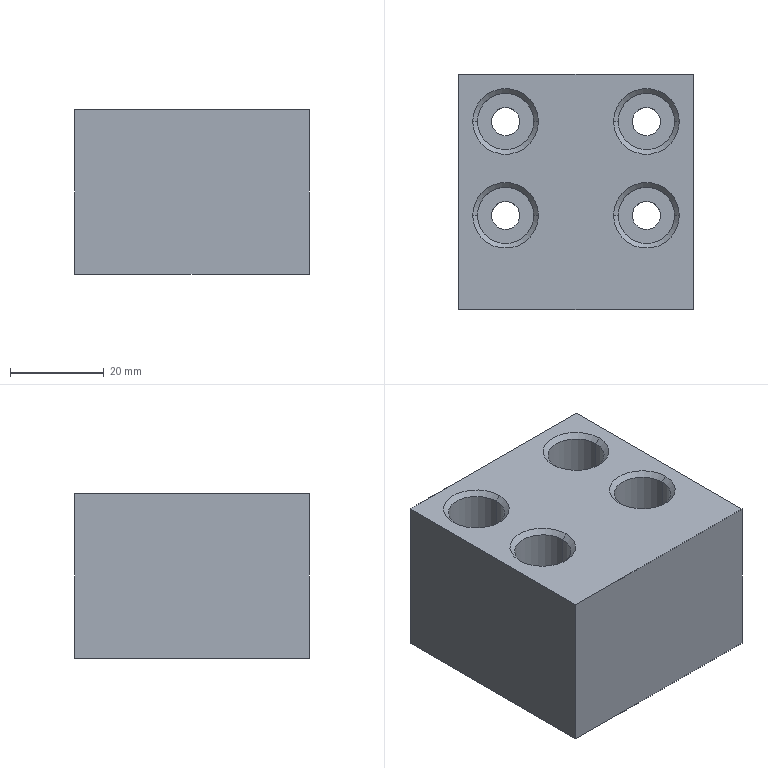Part | STEP file | Stopper | 1 solid | 42 faces | box 50 x 50 x 35 mm | volume 78331 mm3 | cone 16 | cylinder 16 | plane 10 | commonest cylinder face diameters 6 x8 12 x8
STEP:
#1=CARTESIAN_POINT('',(6.228,-22.942,1.));
#2=VERTEX_POINT('',#1);
#3=CARTESIAN_POINT('',(0.2277,-22.942,1.));
#4=VERTEX_POINT('',#3);
#5=CARTESIAN_POINT('',(3.228,-22.942,1.));
#6=DIRECTION('',(0.,0.,-1.));
#7=DIRECTION('',(-1.,0.,0.));
#8=AXIS2_PLACEMENT_3D('',#5,#6,#7);
#9=CIRCLE('',#8,3.);
#10=EDGE_CURVE('',#2,#4,#9,.T.);
#11=ORIENTED_EDGE('',*,*,#10,.F.);
#12=CARTESIAN_POINT('',(7.228,-22.942,0.));
#13=VERTEX_POINT('',#12);
#14=CARTESIAN_POINT('',(7.228,-22.942,0.));
#15=DIRECTION('',(0.7071,0.,-0.7071));
#16=VECTOR('',#15,1000.);
#17=LINE('',#14,#16);
#18=EDGE_CURVE('',#2,#13,#17,.T.);
#19=ORIENTED_EDGE('',*,*,#18,.T.);
#20=CARTESIAN_POINT('',(-0.7723,-22.942,0.));
#21=VERTEX_POINT('',#20);
#22=CARTESIAN_POINT('',(3.228,-22.942,0.));
#23=DIRECTION('',(0.,0.,-1.));
#24=DIRECTION('',(-1.,0.,0.));
#25=AXIS2_PLACEMENT_3D('',#22,#23,#24);
#26=CIRCLE('',#25,4.);
#27=EDGE_CURVE('',#13,#21,#26,.T.);
#28=ORIENTED_EDGE('',*,*,#27,.T.);
#29=CARTESIAN_POINT('',(-0.7723,-22.942,0.));
#30=DIRECTION('',(-0.7071,0.,-0.7071));
#31=VECTOR('',#30,1000.);
#32=LINE('',#29,#31);
#33=EDGE_CURVE('',#4,#21,#32,.T.);
#34=ORIENTED_EDGE('',*,*,#33,.F.);
#35=EDGE_LOOP('',(#11,#19,#28,#34));
#36=FACE_OUTER_BOUND('',#35,.T.);
#37=CARTESIAN_POINT('',(3.228,-22.942,0.));
#38=DIRECTION('',(0.,0.,-1.));
#39=DIRECTION('',(-1.,0.,0.));
#40=AXIS2_PLACEMENT_3D('',#37,#38,#39);
#41=CONICAL_SURFACE('',#40,4.,0.7854);
#42=ADVANCED_FACE('',(#36),#41,.F.);
#43=CARTESIAN_POINT('',(-23.772,-22.942,1.));
#44=VERTEX_POINT('',#43);
#45=CARTESIAN_POINT('',(-29.772,-22.942,1.));
#46=VERTEX_POINT('',#45);
#47=CARTESIAN_POINT('',(-26.772,-22.942,1.));
#48=DIRECTION('',(0.,0.,-1.));
#49=DIRECTION('',(-1.,0.,0.));
#50=AXIS2_PLACEMENT_3D('',#47,#48,#49);
#51=CIRCLE('',#50,3.);
#52=EDGE_CURVE('',#44,#46,#51,.T.);
#53=ORIENTED_EDGE('',*,*,#52,.F.);
#54=CARTESIAN_POINT('',(-22.772,-22.942,0.));
#55=VERTEX_POINT('',#54);
#56=CARTESIAN_POINT('',(-22.772,-22.942,0.));
#57=DIRECTION('',(0.7071,0.,-0.7071));
#58=VECTOR('',#57,1000.);
#59=LINE('',#56,#58);
#60=EDGE_CURVE('',#44,#55,#59,.T.);
#61=ORIENTED_EDGE('',*,*,#60,.T.);
#62=CARTESIAN_POINT('',(-30.772,-22.942,0.));
#63=VERTEX_POINT('',#62);
#64=CARTESIAN_POINT('',(-26.772,-22.942,0.));
#65=DIRECTION('',(0.,0.,-1.));
#66=DIRECTION('',(-1.,0.,0.));
#67=AXIS2_PLACEMENT_3D('',#64,#65,#66);
#68=CIRCLE('',#67,4.);
#69=EDGE_CURVE('',#55,#63,#68,.T.);
#70=ORIENTED_EDGE('',*,*,#69,.T.);
#71=CARTESIAN_POINT('',(-30.772,-22.942,0.));
#72=DIRECTION('',(-0.7071,0.,-0.7071));
#73=VECTOR('',#72,1000.);
#74=LINE('',#71,#73);
#75=EDGE_CURVE('',#46,#63,#74,.T.);
#76=ORIENTED_EDGE('',*,*,#75,.F.);
#77=EDGE_LOOP('',(#53,#61,#70,#76));
#78=FACE_OUTER_BOUND('',#77,.T.);
#79=CARTESIAN_POINT('',(-26.772,-22.942,0.));
#80=DIRECTION('',(0.,0.,-1.));
#81=DIRECTION('',(-1.,0.,0.));
#82=AXIS2_PLACEMENT_3D('',#79,#80,#81);
#83=CONICAL_SURFACE('',#82,4.,0.7854);
#84=ADVANCED_FACE('',(#78),#83,.F.);
#85=CARTESIAN_POINT('',(-23.772,-42.942,1.));
#86=VERTEX_POINT('',#85);
#87=CARTESIAN_POINT('',(-29.772,-42.942,1.));
#88=VERTEX_POINT('',#87);
#89=CARTESIAN_POINT('',(-26.772,-42.942,1.));
#90=DIRECTION('',(0.,0.,-1.));
#91=DIRECTION('',(-1.,0.,0.));
#92=AXIS2_PLACEMENT_3D('',#89,#90,#91);
#93=CIRCLE('',#92,3.);
#94=EDGE_CURVE('',#86,#88,#93,.T.);
#95=ORIENTED_EDGE('',*,*,#94,.F.);
#96=CARTESIAN_POINT('',(-22.772,-42.942,0.));
#97=VERTEX_POINT('',#96);
#98=CARTESIAN_POINT('',(-22.772,-42.942,0.));
#99=DIRECTION('',(0.7071,0.,-0.7071));
#100=VECTOR('',#99,1000.);
#101=LINE('',#98,#100);
#102=EDGE_CURVE('',#86,#97,#101,.T.);
#103=ORIENTED_EDGE('',*,*,#102,.T.);
#104=CARTESIAN_POINT('',(-30.772,-42.942,0.));
#105=VERTEX_POINT('',#104);
#106=CARTESIAN_POINT('',(-26.772,-42.942,0.));
#107=DIRECTION('',(0.,0.,-1.));
#108=DIRECTION('',(-1.,0.,0.));
#109=AXIS2_PLACEMENT_3D('',#106,#107,#108);
#110=CIRCLE('',#109,4.);
#111=EDGE_CURVE('',#97,#105,#110,.T.);
#112=ORIENTED_EDGE('',*,*,#111,.T.);
#113=CARTESIAN_POINT('',(-30.772,-42.942,0.));
#114=DIRECTION('',(-0.7071,0.,-0.7071));
#115=VECTOR('',#114,1000.);
#116=LINE('',#113,#115);
#117=EDGE_CURVE('',#88,#105,#116,.T.);
#118=ORIENTED_EDGE('',*,*,#117,.F.);
#119=EDGE_LOOP('',(#95,#103,#112,#118));
#120=FACE_OUTER_BOUND('',#119,.T.);
#121=CARTESIAN_POINT('',(-26.772,-42.942,0.));
#122=DIRECTION('',(0.,0.,-1.));
#123=DIRECTION('',(-1.,0.,0.));
#124=AXIS2_PLACEMENT_3D('',#121,#122,#123);
#125=CONICAL_SURFACE('',#124,4.,0.7854);
#126=ADVANCED_FACE('',(#120),#125,.F.);
#127=CARTESIAN_POINT('',(6.228,-42.942,1.));
#128=VERTEX_POINT('',#127);
#129=CARTESIAN_POINT('',(0.2277,-42.942,1.));
#130=VERTEX_POINT('',#129);
#131=CARTESIAN_POINT('',(3.228,-42.942,1.));
#132=DIRECTION('',(0.,0.,-1.));
#133=DIRECTION('',(-1.,0.,0.));
#134=AXIS2_PLACEMENT_3D('',#131,#132,#133);
#135=CIRCLE('',#134,3.);
#136=EDGE_CURVE('',#128,#130,#135,.T.);
#137=ORIENTED_EDGE('',*,*,#136,.F.);
#138=CARTESIAN_POINT('',(7.228,-42.942,0.));
#139=VERTEX_POINT('',#138);
#140=CARTESIAN_POINT('',(7.228,-42.942,0.));
#141=DIRECTION('',(0.7071,0.,-0.7071));
#142=VECTOR('',#141,1000.);
#143=LINE('',#140,#142);
#144=EDGE_CURVE('',#128,#139,#143,.T.);
#145=ORIENTED_EDGE('',*,*,#144,.T.);
#146=CARTESIAN_POINT('',(-0.7723,-42.942,0.));
#147=VERTEX_POINT('',#146);
#148=CARTESIAN_POINT('',(3.228,-42.942,0.));
#149=DIRECTION('',(0.,0.,-1.));
#150=DIRECTION('',(-1.,0.,0.));
#151=AXIS2_PLACEMENT_3D('',#148,#149,#150);
#152=CIRCLE('',#151,4.);
#153=EDGE_CURVE('',#139,#147,#152,.T.);
#154=ORIENTED_EDGE('',*,*,#153,.T.);
#155=CARTESIAN_POINT('',(-0.7723,-42.942,0.));
#156=DIRECTION('',(-0.7071,0.,-0.7071));
#157=VECTOR('',#156,1000.);
#158=LINE('',#155,#157);
#159=EDGE_CURVE('',#130,#147,#158,.T.);
#160=ORIENTED_EDGE('',*,*,#159,.F.);
#161=EDGE_LOOP('',(#137,#145,#154,#160));
#162=FACE_OUTER_BOUND('',#161,.T.);
#163=CARTESIAN_POINT('',(3.228,-42.942,0.));
#164=DIRECTION('',(0.,0.,-1.));
#165=DIRECTION('',(-1.,0.,0.));
#166=AXIS2_PLACEMENT_3D('',#163,#164,#165);
#167=CONICAL_SURFACE('',#166,4.,0.7854);
#168=ADVANCED_FACE('',(#162),#167,.F.);
#169=CARTESIAN_POINT('',(6.228,-22.942,20.));
#170=VERTEX_POINT('',#169);
#171=CARTESIAN_POINT('',(0.2277,-22.942,20.));
#172=VERTEX_POINT('',#171);
#173=CARTESIAN_POINT('',(3.228,-22.942,20.));
#174=DIRECTION('',(0.,0.,-1.));
#175=DIRECTION('',(-1.,0.,0.));
#176=AXIS2_PLACEMENT_3D('',#173,#174,#175);
#177=CIRCLE('',#176,3.);
#178=EDGE_CURVE('',#170,#172,#177,.T.);
#179=ORIENTED_EDGE('',*,*,#178,.F.);
#180=CARTESIAN_POINT('',(6.228,-22.942,35.));
#181=DIRECTION('',(0.,0.,-1.));
#182=VECTOR('',#181,1000.);
#183=LINE('',#180,#182);
#184=EDGE_CURVE('',#170,#2,#183,.T.);
#185=ORIENTED_EDGE('',*,*,#184,.T.);
#186=ORIENTED_EDGE('',*,*,#10,.T.);
#187=CARTESIAN_POINT('',(0.2277,-22.942,35.));
#188=DIRECTION('',(0.,0.,-1.));
#189=VECTOR('',#188,1000.);
#190=LINE('',#187,#189);
#191=EDGE_CURVE('',#172,#4,#190,.T.);
#192=ORIENTED_EDGE('',*,*,#191,.F.);
#193=EDGE_LOOP('',(#179,#185,#186,#192));
#194=FACE_OUTER_BOUND('',#193,.T.);
#195=CARTESIAN_POINT('',(3.228,-22.942,35.));
#196=DIRECTION('',(0.,0.,-1.));
#197=DIRECTION('',(-1.,0.,0.));
#198=AXIS2_PLACEMENT_3D('',#195,#196,#197);
#199=CYLINDRICAL_SURFACE('',#198,3.);
#200=ADVANCED_FACE('',(#194),#199,.F.);
#201=CARTESIAN_POINT('',(-23.772,-22.942,20.));
#202=VERTEX_POINT('',#201);
#203=CARTESIAN_POINT('',(-29.772,-22.942,20.));
#204=VERTEX_POINT('',#203);
#205=CARTESIAN_POINT('',(-26.772,-22.942,20.));
#206=DIRECTION('',(0.,0.,-1.));
#207=DIRECTION('',(-1.,0.,0.));
#208=AXIS2_PLACEMENT_3D('',#205,#206,#207);
#209=CIRCLE('',#208,3.);
#210=EDGE_CURVE('',#202,#204,#209,.T.);
#211=ORIENTED_EDGE('',*,*,#210,.F.);
#212=CARTESIAN_POINT('',(-23.772,-22.942,35.));
#213=DIRECTION('',(0.,0.,-1.));
#214=VECTOR('',#213,1000.);
#215=LINE('',#212,#214);
#216=EDGE_CURVE('',#202,#44,#215,.T.);
#217=ORIENTED_EDGE('',*,*,#216,.T.);
#218=ORIENTED_EDGE('',*,*,#52,.T.);
#219=CARTESIAN_POINT('',(-29.772,-22.942,35.));
#220=DIRECTION('',(0.,0.,-1.));
#221=VECTOR('',#220,1000.);
#222=LINE('',#219,#221);
#223=EDGE_CURVE('',#204,#46,#222,.T.);
#224=ORIENTED_EDGE('',*,*,#223,.F.);
#225=EDGE_LOOP('',(#211,#217,#218,#224));
#226=FACE_OUTER_BOUND('',#225,.T.);
#227=CARTESIAN_POINT('',(-26.772,-22.942,35.));
#228=DIRECTION('',(0.,0.,-1.));
#229=DIRECTION('',(-1.,0.,0.));
#230=AXIS2_PLACEMENT_3D('',#227,#228,#229);
#231=CYLINDRICAL_SURFACE('',#230,3.);
#232=ADVANCED_FACE('',(#226),#231,.F.);
#233=CARTESIAN_POINT('',(-23.772,-42.942,20.));
#234=VERTEX_POINT('',#233);
#235=CARTESIAN_POINT('',(-29.772,-42.942,20.));
#236=VERTEX_POINT('',#235);
#237=CARTESIAN_POINT('',(-26.772,-42.942,20.));
#238=DIRECTION('',(0.,0.,-1.));
#239=DIRECTION('',(-1.,0.,0.));
#240=AXIS2_PLACEMENT_3D('',#237,#238,#239);
#241=CIRCLE('',#240,3.);
#242=EDGE_CURVE('',#234,#236,#241,.T.);
#243=ORIENTED_EDGE('',*,*,#242,.F.);
#244=CARTESIAN_POINT('',(-23.772,-42.942,35.));
#245=DIRECTION('',(0.,0.,-1.));
#246=VECTOR('',#245,1000.);
#247=LINE('',#244,#246);
#248=EDGE_CURVE('',#234,#86,#247,.T.);
#249=ORIENTED_EDGE('',*,*,#248,.T.);
#250=ORIENTED_EDGE('',*,*,#94,.T.);
#251=CARTESIAN_POINT('',(-29.772,-42.942,35.));
#252=DIRECTION('',(0.,0.,-1.));
#253=VECTOR('',#252,1000.);
#254=LINE('',#251,#253);
#255=EDGE_CURVE('',#236,#88,#254,.T.);
#256=ORIENTED_EDGE('',*,*,#255,.F.);
#257=EDGE_LOOP('',(#243,#249,#250,#256));
#258=FACE_OUTER_BOUND('',#257,.T.);
#259=CARTESIAN_POINT('',(-26.772,-42.942,35.));
#260=DIRECTION('',(0.,0.,-1.));
#261=DIRECTION('',(-1.,0.,0.));
#262=AXIS2_PLACEMENT_3D('',#259,#260,#261);
#263=CYLINDRICAL_SURFACE('',#262,3.);
#264=ADVANCED_FACE('',(#258),#263,.F.);
#265=CARTESIAN_POINT('',(6.228,-42.942,20.));
#266=VERTEX_POINT('',#265);
#267=CARTESIAN_POINT('',(0.2277,-42.942,20.));
#268=VERTEX_POINT('',#267);
#269=CARTESIAN_POINT('',(3.228,-42.942,20.));
#270=DIRECTION('',(0.,0.,-1.));
#271=DIRECTION('',(-1.,0.,0.));
#272=AXIS2_PLACEMENT_3D('',#269,#270,#271);
#273=CIRCLE('',#272,3.);
#274=EDGE_CURVE('',#266,#268,#273,.T.);
#275=ORIENTED_EDGE('',*,*,#274,.F.);
#276=CARTESIAN_POINT('',(6.228,-42.942,35.));
#277=DIRECTION('',(0.,0.,-1.));
#278=VECTOR('',#277,1000.);
#279=LINE('',#276,#278);
#280=EDGE_CURVE('',#266,#128,#279,.T.);
#281=ORIENTED_EDGE('',*,*,#280,.T.);
#282=ORIENTED_EDGE('',*,*,#136,.T.);
#283=CARTESIAN_POINT('',(0.2277,-42.942,35.));
#284=DIRECTION('',(0.,0.,-1.));
#285=VECTOR('',#284,1000.);
#286=LINE('',#283,#285);
#287=EDGE_CURVE('',#268,#130,#286,.T.);
#288=ORIENTED_EDGE('',*,*,#287,.F.);
#289=EDGE_LOOP('',(#275,#281,#282,#288));
#290=FACE_OUTER_BOUND('',#289,.T.);
#291=CARTESIAN_POINT('',(3.228,-42.942,35.));
#292=DIRECTION('',(0.,0.,-1.));
#293=DIRECTION('',(-1.,0.,0.));
#294=AXIS2_PLACEMENT_3D('',#291,#292,#293);
#295=CYLINDRICAL_SURFACE('',#294,3.);
#296=ADVANCED_FACE('',(#290),#295,.F.);
#297=CARTESIAN_POINT('',(-32.772,-22.942,34.));
#298=VERTEX_POINT('',#297);
#299=CARTESIAN_POINT('',(-20.772,-22.942,34.));
#300=VERTEX_POINT('',#299);
#301=CARTESIAN_POINT('',(-26.772,-22.942,34.));
#302=DIRECTION('',(0.,0.,1.));
#303=DIRECTION('',(1.,0.,0.));
#304=AXIS2_PLACEMENT_3D('',#301,#302,#303);
#305=CIRCLE('',#304,6.);
#306=EDGE_CURVE('',#298,#300,#305,.T.);
#307=ORIENTED_EDGE('',*,*,#306,.F.);
#308=CARTESIAN_POINT('',(-33.772,-22.942,35.));
#309=VERTEX_POINT('',#308);
#310=CARTESIAN_POINT('',(-33.772,-22.942,35.));
#311=DIRECTION('',(-0.7071,0.,0.7071));
#312=VECTOR('',#311,1000.);
#313=LINE('',#310,#312);
#314=EDGE_CURVE('',#298,#309,#313,.T.);
#315=ORIENTED_EDGE('',*,*,#314,.T.);
#316=CARTESIAN_POINT('',(-19.772,-22.942,35.));
#317=VERTEX_POINT('',#316);
#318=CARTESIAN_POINT('',(-26.772,-22.942,35.));
#319=DIRECTION('',(0.,0.,-1.));
#320=DIRECTION('',(1.,0.,0.));
#321=AXIS2_PLACEMENT_3D('',#318,#319,#320);
#322=CIRCLE('',#321,7.);
#323=EDGE_CURVE('',#317,#309,#322,.T.);
#324=ORIENTED_EDGE('',*,*,#323,.F.);
#325=CARTESIAN_POINT('',(-19.772,-22.942,35.));
#326=DIRECTION('',(0.7071,0.,0.7071));
#327=VECTOR('',#326,1000.);
#328=LINE('',#325,#327);
#329=EDGE_CURVE('',#300,#317,#328,.T.);
#330=ORIENTED_EDGE('',*,*,#329,.F.);
#331=EDGE_LOOP('',(#307,#315,#324,#330));
#332=FACE_OUTER_BOUND('',#331,.T.);
#333=CARTESIAN_POINT('',(-26.772,-22.942,35.));
#334=DIRECTION('',(0.,0.,1.));
#335=DIRECTION('',(1.,0.,0.));
#336=AXIS2_PLACEMENT_3D('',#333,#334,#335);
#337=CONICAL_SURFACE('',#336,7.,0.7854);
#338=ADVANCED_FACE('',(#332),#337,.F.);
#339=CARTESIAN_POINT('',(-2.772,-22.942,34.));
#340=VERTEX_POINT('',#339);
#341=CARTESIAN_POINT('',(9.228,-22.942,34.));
#342=VERTEX_POINT('',#341);
#343=CARTESIAN_POINT('',(3.228,-22.942,34.));
#344=DIRECTION('',(0.,0.,1.));
#345=DIRECTION('',(1.,0.,0.));
#346=AXIS2_PLACEMENT_3D('',#343,#344,#345);
#347=CIRCLE('',#346,6.);
#348=EDGE_CURVE('',#340,#342,#347,.T.);
#349=ORIENTED_EDGE('',*,*,#348,.F.);
#350=CARTESIAN_POINT('',(-3.772,-22.942,35.));
#351=VERTEX_POINT('',#350);
#352=CARTESIAN_POINT('',(-3.772,-22.942,35.));
#353=DIRECTION('',(-0.7071,0.,0.7071));
#354=VECTOR('',#353,1000.);
#355=LINE('',#352,#354);
#356=EDGE_CURVE('',#340,#351,#355,.T.);
#357=ORIENTED_EDGE('',*,*,#356,.T.);
#358=CARTESIAN_POINT('',(10.228,-22.942,35.));
#359=VERTEX_POINT('',#358);
#360=CARTESIAN_POINT('',(3.228,-22.942,35.));
#361=DIRECTION('',(0.,0.,-1.));
#362=DIRECTION('',(1.,0.,0.));
#363=AXIS2_PLACEMENT_3D('',#360,#361,#362);
#364=CIRCLE('',#363,7.);
#365=EDGE_CURVE('',#359,#351,#364,.T.);
#366=ORIENTED_EDGE('',*,*,#365,.F.);
#367=CARTESIAN_POINT('',(10.228,-22.942,35.));
#368=DIRECTION('',(0.7071,0.,0.7071));
#369=VECTOR('',#368,1000.);
#370=LINE('',#367,#369);
#371=EDGE_CURVE('',#342,#359,#370,.T.);
#372=ORIENTED_EDGE('',*,*,#371,.F.);
#373=EDGE_LOOP('',(#349,#357,#366,#372));
#374=FACE_OUTER_BOUND('',#373,.T.);
#375=CARTESIAN_POINT('',(3.228,-22.942,35.));
#376=DIRECTION('',(0.,0.,1.));
#377=DIRECTION('',(1.,0.,0.));
#378=AXIS2_PLACEMENT_3D('',#375,#376,#377);
#379=CONICAL_SURFACE('',#378,7.,0.7854);
#380=ADVANCED_FACE('',(#374),#379,.F.);
#381=CARTESIAN_POINT('',(-2.772,-42.942,34.));
#382=VERTEX_POINT('',#381);
#383=CARTESIAN_POINT('',(9.228,-42.942,34.));
#384=VERTEX_POINT('',#383);
#385=CARTESIAN_POINT('',(3.228,-42.942,34.));
#386=DIRECTION('',(0.,0.,1.));
#387=DIRECTION('',(1.,0.,0.));
#388=AXIS2_PLACEMENT_3D('',#385,#386,#387);
#389=CIRCLE('',#388,6.);
#390=EDGE_CURVE('',#382,#384,#389,.T.);
#391=ORIENTED_EDGE('',*,*,#390,.F.);
#392=CARTESIAN_POINT('',(-3.772,-42.942,35.));
#393=VERTEX_POINT('',#392);
#394=CARTESIAN_POINT('',(-3.772,-42.942,35.));
#395=DIRECTION('',(-0.7071,0.,0.7071));
#396=VECTOR('',#395,1000.);
#397=LINE('',#394,#396);
#398=EDGE_CURVE('',#382,#393,#397,.T.);
#399=ORIENTED_EDGE('',*,*,#398,.T.);
#400=CARTESIAN_POINT('',(10.228,-42.942,35.));
#401=VERTEX_POINT('',#400);
#402=CARTESIAN_POINT('',(3.228,-42.942,35.));
#403=DIRECTION('',(0.,0.,-1.));
#404=DIRECTION('',(1.,0.,0.));
#405=AXIS2_PLACEMENT_3D('',#402,#403,#404);
#406=CIRCLE('',#405,7.);
#407=EDGE_CURVE('',#401,#393,#406,.T.);
#408=ORIENTED_EDGE('',*,*,#407,.F.);
#409=CARTESIAN_POINT('',(10.228,-42.942,35.));
#410=DIRECTION('',(0.7071,0.,0.7071));
#411=VECTOR('',#410,1000.);
#412=LINE('',#409,#411);
#413=EDGE_CURVE('',#384,#401,#412,.T.);
#414=ORIENTED_EDGE('',*,*,#413,.F.);
#415=EDGE_LOOP('',(#391,#399,#408,#414));
#416=FACE_OUTER_BOUND('',#415,.T.);
#417=CARTESIAN_POINT('',(3.228,-42.942,35.));
#418=DIRECTION('',(0.,0.,1.));
#419=DIRECTION('',(1.,0.,0.));
#420=AXIS2_PLACEMENT_3D('',#417,#418,#419);
#421=CONICAL_SURFACE('',#420,7.,0.7854);
#422=ADVANCED_FACE('',(#416),#421,.F.);
#423=CARTESIAN_POINT('',(-32.772,-42.942,34.));
#424=VERTEX_POINT('',#423);
#425=CARTESIAN_POINT('',(-20.772,-42.942,34.));
#426=VERTEX_POINT('',#425);
#427=CARTESIAN_POINT('',(-26.772,-42.942,34.));
#428=DIRECTION('',(0.,0.,1.));
#429=DIRECTION('',(1.,0.,0.));
#430=AXIS2_PLACEMENT_3D('',#427,#428,#429);
#431=CIRCLE('',#430,6.);
#432=EDGE_CURVE('',#424,#426,#431,.T.);
#433=ORIENTED_EDGE('',*,*,#432,.F.);
#434=CARTESIAN_POINT('',(-33.772,-42.942,35.));
#435=VERTEX_POINT('',#434);
#436=CARTESIAN_POINT('',(-33.772,-42.942,35.));
#437=DIRECTION('',(-0.7071,0.,0.7071));
#438=VECTOR('',#437,1000.);
#439=LINE('',#436,#438);
#440=EDGE_CURVE('',#424,#435,#439,.T.);
#441=ORIENTED_EDGE('',*,*,#440,.T.);
#442=CARTESIAN_POINT('',(-19.772,-42.942,35.));
#443=VERTEX_POINT('',#442);
#444=CARTESIAN_POINT('',(-26.772,-42.942,35.));
#445=DIRECTION('',(0.,0.,-1.));
#446=DIRECTION('',(1.,0.,0.));
#447=AXIS2_PLACEMENT_3D('',#444,#445,#446);
#448=CIRCLE('',#447,7.);
#449=EDGE_CURVE('',#443,#435,#448,.T.);
#450=ORIENTED_EDGE('',*,*,#449,.F.);
#451=CARTESIAN_POINT('',(-19.772,-42.942,35.));
#452=DIRECTION('',(0.7071,0.,0.7071));
#453=VECTOR('',#452,1000.);
#454=LINE('',#451,#453);
#455=EDGE_CURVE('',#426,#443,#454,.T.);
#456=ORIENTED_EDGE('',*,*,#455,.F.);
#457=EDGE_LOOP('',(#433,#441,#450,#456));
#458=FACE_OUTER_BOUND('',#457,.T.);
#459=CARTESIAN_POINT('',(-26.772,-42.942,35.));
#460=DIRECTION('',(0.,0.,1.));
#461=DIRECTION('',(1.,0.,0.));
#462=AXIS2_PLACEMENT_3D('',#459,#460,#461);
#463=CONICAL_SURFACE('',#462,7.,0.7854);
#464=ADVANCED_FACE('',(#458),#463,.F.);
#465=CARTESIAN_POINT('',(-32.772,-22.942,20.));
#466=VERTEX_POINT('',#465);
#467=CARTESIAN_POINT('',(-20.772,-22.942,20.));
#468=VERTEX_POINT('',#467);
#469=CARTESIAN_POINT('',(-26.772,-22.942,20.));
#470=DIRECTION('',(0.,0.,1.));
#471=DIRECTION('',(1.,0.,0.));
#472=AXIS2_PLACEMENT_3D('',#469,#470,#471);
#473=CIRCLE('',#472,6.);
#474=EDGE_CURVE('',#466,#468,#473,.T.);
#475=ORIENTED_EDGE('',*,*,#474,.F.);
#476=CARTESIAN_POINT('',(-32.772,-22.942,20.));
#477=DIRECTION('',(0.,0.,1.));
#478=VECTOR('',#477,1000.);
#479=LINE('',#476,#478);
#480=EDGE_CURVE('',#466,#298,#479,.T.);
#481=ORIENTED_EDGE('',*,*,#480,.T.);
#482=ORIENTED_EDGE('',*,*,#306,.T.);
#483=CARTESIAN_POINT('',(-20.772,-22.942,20.));
#484=DIRECTION('',(0.,0.,1.));
#485=VECTOR('',#484,1000.);
#486=LINE('',#483,#485);
#487=EDGE_CURVE('',#468,#300,#486,.T.);
#488=ORIENTED_EDGE('',*,*,#487,.F.);
#489=EDGE_LOOP('',(#475,#481,#482,#488));
#490=FACE_OUTER_BOUND('',#489,.T.);
#491=CARTESIAN_POINT('',(-26.772,-22.942,20.));
#492=DIRECTION('',(0.,0.,1.));
#493=DIRECTION('',(1.,0.,0.));
#494=AXIS2_PLACEMENT_3D('',#491,#492,#493);
#495=CYLINDRICAL_SURFACE('',#494,6.);
#496=ADVANCED_FACE('',(#490),#495,.F.);
#497=CARTESIAN_POINT('',(-2.772,-22.942,20.));
#498=VERTEX_POINT('',#497);
#499=CARTESIAN_POINT('',(9.228,-22.942,20.));
#500=VERTEX_POINT('',#499);
#501=CARTESIAN_POINT('',(3.228,-22.942,20.));
#502=DIRECTION('',(0.,0.,1.));
#503=DIRECTION('',(1.,0.,0.));
#504=AXIS2_PLACEMENT_3D('',#501,#502,#503);
#505=CIRCLE('',#504,6.);
#506=EDGE_CURVE('',#498,#500,#505,.T.);
#507=ORIENTED_EDGE('',*,*,#506,.F.);
#508=CARTESIAN_POINT('',(-2.772,-22.942,20.));
#509=DIRECTION('',(0.,0.,1.));
#510=VECTOR('',#509,1000.);
#511=LINE('',#508,#510);
#512=EDGE_CURVE('',#498,#340,#511,.T.);
#513=ORIENTED_EDGE('',*,*,#512,.T.);
#514=ORIENTED_EDGE('',*,*,#348,.T.);
#515=CARTESIAN_POINT('',(9.228,-22.942,20.));
#516=DIRECTION('',(0.,0.,1.));
#517=VECTOR('',#516,1000.);
#518=LINE('',#515,#517);
#519=EDGE_CURVE('',#500,#342,#518,.T.);
#520=ORIENTED_EDGE('',*,*,#519,.F.);
#521=EDGE_LOOP('',(#507,#513,#514,#520));
#522=FACE_OUTER_BOUND('',#521,.T.);
#523=CARTESIAN_POINT('',(3.228,-22.942,20.));
#524=DIRECTION('',(0.,0.,1.));
#525=DIRECTION('',(1.,0.,0.));
#526=AXIS2_PLACEMENT_3D('',#523,#524,#525);
#527=CYLINDRICAL_SURFACE('',#526,6.);
#528=ADVANCED_FACE('',(#522),#527,.F.);
#529=CARTESIAN_POINT('',(-2.772,-42.942,20.));
#530=VERTEX_POINT('',#529);
#531=CARTESIAN_POINT('',(9.228,-42.942,20.));
#532=VERTEX_POINT('',#531);
#533=CARTESIAN_POINT('',(3.228,-42.942,20.));
#534=DIRECTION('',(0.,0.,1.));
#535=DIRECTION('',(1.,0.,0.));
#536=AXIS2_PLACEMENT_3D('',#533,#534,#535);
#537=CIRCLE('',#536,6.);
#538=EDGE_CURVE('',#530,#532,#537,.T.);
#539=ORIENTED_EDGE('',*,*,#538,.F.);
#540=CARTESIAN_POINT('',(-2.772,-42.942,20.));
#541=DIRECTION('',(0.,0.,1.));
#542=VECTOR('',#541,1000.);
#543=LINE('',#540,#542);
#544=EDGE_CURVE('',#530,#382,#543,.T.);
#545=ORIENTED_EDGE('',*,*,#544,.T.);
#546=ORIENTED_EDGE('',*,*,#390,.T.);
#547=CARTESIAN_POINT('',(9.228,-42.942,20.));
#548=DIRECTION('',(0.,0.,1.));
#549=VECTOR('',#548,1000.);
#550=LINE('',#547,#549);
#551=EDGE_CURVE('',#532,#384,#550,.T.);
#552=ORIENTED_EDGE('',*,*,#551,.F.);
#553=EDGE_LOOP('',(#539,#545,#546,#552));
#554=FACE_OUTER_BOUND('',#553,.T.);
#555=CARTESIAN_POINT('',(3.228,-42.942,20.));
#556=DIRECTION('',(0.,0.,1.));
#557=DIRECTION('',(1.,0.,0.));
#558=AXIS2_PLACEMENT_3D('',#555,#556,#557);
#559=CYLINDRICAL_SURFACE('',#558,6.);
#560=ADVANCED_FACE('',(#554),#559,.F.);
#561=CARTESIAN_POINT('',(-32.772,-42.942,20.));
#562=VERTEX_POINT('',#561);
#563=CARTESIAN_POINT('',(-20.772,-42.942,20.));
#564=VERTEX_POINT('',#563);
#565=CARTESIAN_POINT('',(-26.772,-42.942,20.));
#566=DIRECTION('',(0.,0.,1.));
#567=DIRECTION('',(1.,0.,0.));
#568=AXIS2_PLACEMENT_3D('',#565,#566,#567);
#569=CIRCLE('',#568,6.);
#570=EDGE_CURVE('',#562,#564,#569,.T.);
#571=ORIENTED_EDGE('',*,*,#570,.F.);
#572=CARTESIAN_POINT('',(-32.772,-42.942,20.));
#573=DIRECTION('',(0.,0.,1.));
#574=VECTOR('',#573,1000.);
#575=LINE('',#572,#574);
#576=EDGE_CURVE('',#562,#424,#575,.T.);
#577=ORIENTED_EDGE('',*,*,#576,.T.);
#578=ORIENTED_EDGE('',*,*,#432,.T.);
#579=CARTESIAN_POINT('',(-20.772,-42.942,20.));
#580=DIRECTION('',(0.,0.,1.));
#581=VECTOR('',#580,1000.);
#582=LINE('',#579,#581);
#583=EDGE_CURVE('',#564,#426,#582,.T.);
#584=ORIENTED_EDGE('',*,*,#583,.F.);
#585=EDGE_LOOP('',(#571,#577,#578,#584));
#586=FACE_OUTER_BOUND('',#585,.T.);
#587=CARTESIAN_POINT('',(-26.772,-42.942,20.));
#588=DIRECTION('',(0.,0.,1.));
#589=DIRECTION('',(1.,0.,0.));
#590=AXIS2_PLACEMENT_3D('',#587,#588,#589);
#591=CYLINDRICAL_SURFACE('',#590,6.);
#592=ADVANCED_FACE('',(#586),#591,.F.);
#593=CARTESIAN_POINT('',(13.228,-12.942,0.));
#594=VERTEX_POINT('',#593);
#595=CARTESIAN_POINT('',(-36.772,-12.942,0.));
#596=VERTEX_POINT('',#595);
#597=CARTESIAN_POINT('',(-36.772,-12.942,0.));
#598=DIRECTION('',(-1.,0.,0.));
#599=VECTOR('',#598,1000.);
#600=LINE('',#597,#599);
#601=EDGE_CURVE('',#594,#596,#600,.T.);
#602=ORIENTED_EDGE('',*,*,#601,.F.);
#603=CARTESIAN_POINT('',(13.228,-62.942,0.));
#604=VERTEX_POINT('',#603);
#605=CARTESIAN_POINT('',(13.228,-62.942,0.));
#606=DIRECTION('',(0.,1.,0.));
#607=VECTOR('',#606,1000.);
#608=LINE('',#605,#607);
#609=EDGE_CURVE('',#604,#594,#608,.T.);
#610=ORIENTED_EDGE('',*,*,#609,.F.);
#611=CARTESIAN_POINT('',(-36.772,-62.942,0.));
#612=VERTEX_POINT('',#611);
#613=CARTESIAN_POINT('',(-36.772,-62.942,0.));
#614=DIRECTION('',(1.,0.,0.));
#615=VECTOR('',#614,1000.);
#616=LINE('',#613,#615);
#617=EDGE_CURVE('',#612,#604,#616,.T.);
#618=ORIENTED_EDGE('',*,*,#617,.F.);
#619=CARTESIAN_POINT('',(-36.772,-62.942,0.));
#620=DIRECTION('',(0.,-1.,0.));
#621=VECTOR('',#620,1000.);
#622=LINE('',#619,#621);
#623=EDGE_CURVE('',#596,#612,#622,.T.);
#624=ORIENTED_EDGE('',*,*,#623,.F.);
#625=EDGE_LOOP('',(#602,#610,#618,#624));
#626=FACE_OUTER_BOUND('',#625,.T.);
#627=CARTESIAN_POINT('',(3.228,-22.942,0.));
#628=DIRECTION('',(0.,0.,-1.));
#629=DIRECTION('',(-1.,0.,0.));
#630=AXIS2_PLACEMENT_3D('',#627,#628,#629);
#631=CIRCLE('',#630,4.);
#632=EDGE_CURVE('',#21,#13,#631,.T.);
#633=ORIENTED_EDGE('',*,*,#632,.F.);
#634=ORIENTED_EDGE('',*,*,#27,.F.);
#635=EDGE_LOOP('',(#633,#634));
#636=FACE_BOUND('',#635,.T.);
#637=CARTESIAN_POINT('',(-26.772,-22.942,0.));
#638=DIRECTION('',(0.,0.,-1.));
#639=DIRECTION('',(-1.,0.,0.));
#640=AXIS2_PLACEMENT_3D('',#637,#638,#639);
#641=CIRCLE('',#640,4.);
#642=EDGE_CURVE('',#63,#55,#641,.T.);
#643=ORIENTED_EDGE('',*,*,#642,.F.);
#644=ORIENTED_EDGE('',*,*,#69,.F.);
#645=EDGE_LOOP('',(#643,#644));
#646=FACE_BOUND('',#645,.T.);
#647=CARTESIAN_POINT('',(-26.772,-42.942,0.));
#648=DIRECTION('',(0.,0.,-1.));
#649=DIRECTION('',(-1.,0.,0.));
#650=AXIS2_PLACEMENT_3D('',#647,#648,#649);
#651=CIRCLE('',#650,4.);
#652=EDGE_CURVE('',#105,#97,#651,.T.);
#653=ORIENTED_EDGE('',*,*,#652,.F.);
#654=ORIENTED_EDGE('',*,*,#111,.F.);
#655=EDGE_LOOP('',(#653,#654));
#656=FACE_BOUND('',#655,.T.);
#657=CARTESIAN_POINT('',(3.228,-42.942,0.));
#658=DIRECTION('',(0.,0.,-1.));
#659=DIRECTION('',(-1.,0.,0.));
#660=AXIS2_PLACEMENT_3D('',#657,#658,#659);
#661=CIRCLE('',#660,4.);
#662=EDGE_CURVE('',#147,#139,#661,.T.);
#663=ORIENTED_EDGE('',*,*,#662,.F.);
#664=ORIENTED_EDGE('',*,*,#153,.F.);
#665=EDGE_LOOP('',(#663,#664));
#666=FACE_BOUND('',#665,.T.);
#667=CARTESIAN_POINT('',(-36.772,-62.942,0.));
#668=DIRECTION('',(0.,0.,1.));
#669=DIRECTION('',(1.,0.,0.));
#670=AXIS2_PLACEMENT_3D('',#667,#668,#669);
#671=PLANE('',#670);
#672=ADVANCED_FACE('',(#626,#636,#646,#656,#666),#671,.F.);
#673=CARTESIAN_POINT('',(-36.772,-62.942,35.));
#674=VERTEX_POINT('',#673);
#675=CARTESIAN_POINT('',(-36.772,-62.942,35.));
#676=DIRECTION('',(0.,0.,-1.));
#677=VECTOR('',#676,1000.);
#678=LINE('',#675,#677);
#679=EDGE_CURVE('',#674,#612,#678,.T.);
#680=ORIENTED_EDGE('',*,*,#679,.F.);
#681=CARTESIAN_POINT('',(-36.772,-12.942,35.));
#682=VERTEX_POINT('',#681);
#683=CARTESIAN_POINT('',(-36.772,-12.942,35.));
#684=DIRECTION('',(0.,-1.,0.));
#685=VECTOR('',#684,1000.);
#686=LINE('',#683,#685);
#687=EDGE_CURVE('',#682,#674,#686,.T.);
#688=ORIENTED_EDGE('',*,*,#687,.F.);
#689=CARTESIAN_POINT('',(-36.772,-12.942,35.));
#690=DIRECTION('',(0.,0.,1.));
#691=VECTOR('',#690,1000.);
#692=LINE('',#689,#691);
#693=EDGE_CURVE('',#596,#682,#692,.T.);
#694=ORIENTED_EDGE('',*,*,#693,.F.);
#695=ORIENTED_EDGE('',*,*,#623,.T.);
#696=EDGE_LOOP('',(#680,#688,#694,#695));
#697=FACE_OUTER_BOUND('',#696,.T.);
#698=CARTESIAN_POINT('',(-36.772,-12.942,35.));
#699=DIRECTION('',(1.,0.,0.));
#700=DIRECTION('',(0.,0.,-1.));
#701=AXIS2_PLACEMENT_3D('',#698,#699,#700);
#702=PLANE('',#701);
#703=ADVANCED_FACE('',(#697),#702,.F.);
#704=ORIENTED_EDGE('',*,*,#693,.T.);
#705=CARTESIAN_POINT('',(13.228,-12.942,35.));
#706=VERTEX_POINT('',#705);
#707=CARTESIAN_POINT('',(-36.772,-12.942,35.));
#708=DIRECTION('',(-1.,0.,0.));
#709=VECTOR('',#708,1000.);
#710=LINE('',#707,#709);
#711=EDGE_CURVE('',#706,#682,#710,.T.);
#712=ORIENTED_EDGE('',*,*,#711,.F.);
#713=CARTESIAN_POINT('',(13.228,-12.942,35.));
#714=DIRECTION('',(0.,0.,1.));
#715=VECTOR('',#714,1000.);
#716=LINE('',#713,#715);
#717=EDGE_CURVE('',#594,#706,#716,.T.);
#718=ORIENTED_EDGE('',*,*,#717,.F.);
#719=ORIENTED_EDGE('',*,*,#601,.T.);
#720=EDGE_LOOP('',(#704,#712,#718,#719));
#721=FACE_OUTER_BOUND('',#720,.T.);
#722=CARTESIAN_POINT('',(-36.772,-12.942,35.));
#723=DIRECTION('',(0.,-1.,0.));
#724=DIRECTION('',(0.,0.,-1.));
#725=AXIS2_PLACEMENT_3D('',#722,#723,#724);
#726=PLANE('',#725);
#727=ADVANCED_FACE('',(#721),#726,.F.);
#728=ORIENTED_EDGE('',*,*,#717,.T.);
#729=CARTESIAN_POINT('',(13.228,-62.942,35.));
#730=VERTEX_POINT('',#729);
#731=CARTESIAN_POINT('',(13.228,-12.942,35.));
#732=DIRECTION('',(0.,1.,0.));
#733=VECTOR('',#732,1000.);
#734=LINE('',#731,#733);
#735=EDGE_CURVE('',#730,#706,#734,.T.);
#736=ORIENTED_EDGE('',*,*,#735,.F.);
#737=CARTESIAN_POINT('',(13.228,-62.942,35.));
#738=DIRECTION('',(0.,0.,1.));
#739=VECTOR('',#738,1000.);
#740=LINE('',#737,#739);
#741=EDGE_CURVE('',#604,#730,#740,.T.);
#742=ORIENTED_EDGE('',*,*,#741,.F.);
#743=ORIENTED_EDGE('',*,*,#609,.T.);
#744=EDGE_LOOP('',(#728,#736,#742,#743));
#745=FACE_OUTER_BOUND('',#744,.T.);
#746=CARTESIAN_POINT('',(13.228,-12.942,35.));
#747=DIRECTION('',(-1.,0.,0.));
#748=DIRECTION('',(0.,0.,1.));
#749=AXIS2_PLACEMENT_3D('',#746,#747,#748);
#750=PLANE('',#749);
#751=ADVANCED_FACE('',(#745),#750,.F.);
#752=ORIENTED_EDGE('',*,*,#741,.T.);
#753=CARTESIAN_POINT('',(-36.772,-62.942,35.));
#754=DIRECTION('',(1.,0.,0.));
#755=VECTOR('',#754,1000.);
#756=LINE('',#753,#755);
#757=EDGE_CURVE('',#674,#730,#756,.T.);
#758=ORIENTED_EDGE('',*,*,#757,.F.);
#759=ORIENTED_EDGE('',*,*,#679,.T.);
#760=ORIENTED_EDGE('',*,*,#617,.T.);
#761=EDGE_LOOP('',(#752,#758,#759,#760));
#762=FACE_OUTER_BOUND('',#761,.T.);
#763=CARTESIAN_POINT('',(-36.772,-62.942,35.));
#764=DIRECTION('',(0.,1.,0.));
#765=DIRECTION('',(0.,0.,1.));
#766=AXIS2_PLACEMENT_3D('',#763,#764,#765);
#767=PLANE('',#766);
#768=ADVANCED_FACE('',(#762),#767,.F.);
#769=ORIENTED_EDGE('',*,*,#18,.F.);
#770=CARTESIAN_POINT('',(3.228,-22.942,1.));
#771=DIRECTION('',(0.,0.,-1.));
#772=DIRECTION('',(-1.,0.,0.));
#773=AXIS2_PLACEMENT_3D('',#770,#771,#772);
#774=CIRCLE('',#773,3.);
#775=EDGE_CURVE('',#4,#2,#774,.T.);
#776=ORIENTED_EDGE('',*,*,#775,.F.);
#777=ORIENTED_EDGE('',*,*,#33,.T.);
#778=ORIENTED_EDGE('',*,*,#632,.T.);
#779=EDGE_LOOP('',(#769,#776,#777,#778));
#780=FACE_OUTER_BOUND('',#779,.T.);
#781=CARTESIAN_POINT('',(3.228,-22.942,0.));
#782=DIRECTION('',(0.,0.,-1.));
#783=DIRECTION('',(-1.,0.,0.));
#784=AXIS2_PLACEMENT_3D('',#781,#782,#783);
#785=CONICAL_SURFACE('',#784,4.,0.7854);
#786=ADVANCED_FACE('',(#780),#785,.F.);
#787=ORIENTED_EDGE('',*,*,#60,.F.);
#788=CARTESIAN_POINT('',(-26.772,-22.942,1.));
#789=DIRECTION('',(0.,0.,-1.));
#790=DIRECTION('',(-1.,0.,0.));
#791=AXIS2_PLACEMENT_3D('',#788,#789,#790);
#792=CIRCLE('',#791,3.);
#793=EDGE_CURVE('',#46,#44,#792,.T.);
#794=ORIENTED_EDGE('',*,*,#793,.F.);
#795=ORIENTED_EDGE('',*,*,#75,.T.);
#796=ORIENTED_EDGE('',*,*,#642,.T.);
#797=EDGE_LOOP('',(#787,#794,#795,#796));
#798=FACE_OUTER_BOUND('',#797,.T.);
#799=CARTESIAN_POINT('',(-26.772,-22.942,0.));
#800=DIRECTION('',(0.,0.,-1.));
#801=DIRECTION('',(-1.,0.,0.));
#802=AXIS2_PLACEMENT_3D('',#799,#800,#801);
#803=CONICAL_SURFACE('',#802,4.,0.7854);
#804=ADVANCED_FACE('',(#798),#803,.F.);
#805=ORIENTED_EDGE('',*,*,#102,.F.);
#806=CARTESIAN_POINT('',(-26.772,-42.942,1.));
#807=DIRECTION('',(0.,0.,-1.));
#808=DIRECTION('',(-1.,0.,0.));
#809=AXIS2_PLACEMENT_3D('',#806,#807,#808);
#810=CIRCLE('',#809,3.);
#811=EDGE_CURVE('',#88,#86,#810,.T.);
#812=ORIENTED_EDGE('',*,*,#811,.F.);
#813=ORIENTED_EDGE('',*,*,#117,.T.);
#814=ORIENTED_EDGE('',*,*,#652,.T.);
#815=EDGE_LOOP('',(#805,#812,#813,#814));
#816=FACE_OUTER_BOUND('',#815,.T.);
#817=CARTESIAN_POINT('',(-26.772,-42.942,0.));
#818=DIRECTION('',(0.,0.,-1.));
#819=DIRECTION('',(-1.,0.,0.));
#820=AXIS2_PLACEMENT_3D('',#817,#818,#819);
#821=CONICAL_SURFACE('',#820,4.,0.7854);
#822=ADVANCED_FACE('',(#816),#821,.F.);
#823=ORIENTED_EDGE('',*,*,#144,.F.);
#824=CARTESIAN_POINT('',(3.228,-42.942,1.));
#825=DIRECTION('',(0.,0.,-1.));
#826=DIRECTION('',(-1.,0.,0.));
#827=AXIS2_PLACEMENT_3D('',#824,#825,#826);
#828=CIRCLE('',#827,3.);
#829=EDGE_CURVE('',#130,#128,#828,.T.);
#830=ORIENTED_EDGE('',*,*,#829,.F.);
#831=ORIENTED_EDGE('',*,*,#159,.T.);
#832=ORIENTED_EDGE('',*,*,#662,.T.);
#833=EDGE_LOOP('',(#823,#830,#831,#832));
#834=FACE_OUTER_BOUND('',#833,.T.);
#835=CARTESIAN_POINT('',(3.228,-42.942,0.));
#836=DIRECTION('',(0.,0.,-1.));
#837=DIRECTION('',(-1.,0.,0.));
#838=AXIS2_PLACEMENT_3D('',#835,#836,#837);
#839=CONICAL_SURFACE('',#838,4.,0.7854);
#840=ADVANCED_FACE('',(#834),#839,.F.);
#841=ORIENTED_EDGE('',*,*,#735,.T.);
#842=ORIENTED_EDGE('',*,*,#711,.T.);
#843=ORIENTED_EDGE('',*,*,#687,.T.);
#844=ORIENTED_EDGE('',*,*,#757,.T.);
#845=EDGE_LOOP('',(#841,#842,#843,#844));
#846=FACE_OUTER_BOUND('',#845,.T.);
#847=ORIENTED_EDGE('',*,*,#323,.T.);
#848=CARTESIAN_POINT('',(-26.772,-22.942,35.));
#849=DIRECTION('',(0.,0.,-1.));
#850=DIRECTION('',(1.,0.,0.));
#851=AXIS2_PLACEMENT_3D('',#848,#849,#850);
#852=CIRCLE('',#851,7.);
#853=EDGE_CURVE('',#309,#317,#852,.T.);
#854=ORIENTED_EDGE('',*,*,#853,.T.);
#855=EDGE_LOOP('',(#847,#854));
#856=FACE_BOUND('',#855,.T.);
#857=ORIENTED_EDGE('',*,*,#365,.T.);
#858=CARTESIAN_POINT('',(3.228,-22.942,35.));
#859=DIRECTION('',(0.,0.,-1.));
#860=DIRECTION('',(1.,0.,0.));
#861=AXIS2_PLACEMENT_3D('',#858,#859,#860);
#862=CIRCLE('',#861,7.);
#863=EDGE_CURVE('',#351,#359,#862,.T.);
#864=ORIENTED_EDGE('',*,*,#863,.T.);
#865=EDGE_LOOP('',(#857,#864));
#866=FACE_BOUND('',#865,.T.);
#867=ORIENTED_EDGE('',*,*,#407,.T.);
#868=CARTESIAN_POINT('',(3.228,-42.942,35.));
#869=DIRECTION('',(0.,0.,-1.));
#870=DIRECTION('',(1.,0.,0.));
#871=AXIS2_PLACEMENT_3D('',#868,#869,#870);
#872=CIRCLE('',#871,7.);
#873=EDGE_CURVE('',#393,#401,#872,.T.);
#874=ORIENTED_EDGE('',*,*,#873,.T.);
#875=EDGE_LOOP('',(#867,#874));
#876=FACE_BOUND('',#875,.T.);
#877=ORIENTED_EDGE('',*,*,#449,.T.);
#878=CARTESIAN_POINT('',(-26.772,-42.942,35.));
#879=DIRECTION('',(0.,0.,-1.));
#880=DIRECTION('',(1.,0.,0.));
#881=AXIS2_PLACEMENT_3D('',#878,#879,#880);
#882=CIRCLE('',#881,7.);
#883=EDGE_CURVE('',#435,#443,#882,.T.);
#884=ORIENTED_EDGE('',*,*,#883,.T.);
#885=EDGE_LOOP('',(#877,#884));
#886=FACE_BOUND('',#885,.T.);
#887=CARTESIAN_POINT('',(-36.772,-62.942,35.));
#888=DIRECTION('',(0.,0.,1.));
#889=DIRECTION('',(1.,0.,0.));
#890=AXIS2_PLACEMENT_3D('',#887,#888,#889);
#891=PLANE('',#890);
#892=ADVANCED_FACE('',(#846,#856,#866,#876,#886),#891,.T.);
#893=ORIENTED_EDGE('',*,*,#184,.F.);
#894=CARTESIAN_POINT('',(3.228,-22.942,20.));
#895=DIRECTION('',(0.,0.,-1.));
#896=DIRECTION('',(-1.,0.,0.));
#897=AXIS2_PLACEMENT_3D('',#894,#895,#896);
#898=CIRCLE('',#897,3.);
#899=EDGE_CURVE('',#172,#170,#898,.T.);
#900=ORIENTED_EDGE('',*,*,#899,.F.);
#901=ORIENTED_EDGE('',*,*,#191,.T.);
#902=ORIENTED_EDGE('',*,*,#775,.T.);
#903=EDGE_LOOP('',(#893,#900,#901,#902));
#904=FACE_OUTER_BOUND('',#903,.T.);
#905=CARTESIAN_POINT('',(3.228,-22.942,35.));
#906=DIRECTION('',(0.,0.,-1.));
#907=DIRECTION('',(-1.,0.,0.));
#908=AXIS2_PLACEMENT_3D('',#905,#906,#907);
#909=CYLINDRICAL_SURFACE('',#908,3.);
#910=ADVANCED_FACE('',(#904),#909,.F.);
#911=ORIENTED_EDGE('',*,*,#216,.F.);
#912=CARTESIAN_POINT('',(-26.772,-22.942,20.));
#913=DIRECTION('',(0.,0.,-1.));
#914=DIRECTION('',(-1.,0.,0.));
#915=AXIS2_PLACEMENT_3D('',#912,#913,#914);
#916=CIRCLE('',#915,3.);
#917=EDGE_CURVE('',#204,#202,#916,.T.);
#918=ORIENTED_EDGE('',*,*,#917,.F.);
#919=ORIENTED_EDGE('',*,*,#223,.T.);
#920=ORIENTED_EDGE('',*,*,#793,.T.);
#921=EDGE_LOOP('',(#911,#918,#919,#920));
#922=FACE_OUTER_BOUND('',#921,.T.);
#923=CARTESIAN_POINT('',(-26.772,-22.942,35.));
#924=DIRECTION('',(0.,0.,-1.));
#925=DIRECTION('',(-1.,0.,0.));
#926=AXIS2_PLACEMENT_3D('',#923,#924,#925);
#927=CYLINDRICAL_SURFACE('',#926,3.);
#928=ADVANCED_FACE('',(#922),#927,.F.);
#929=ORIENTED_EDGE('',*,*,#248,.F.);
#930=CARTESIAN_POINT('',(-26.772,-42.942,20.));
#931=DIRECTION('',(0.,0.,-1.));
#932=DIRECTION('',(-1.,0.,0.));
#933=AXIS2_PLACEMENT_3D('',#930,#931,#932);
#934=CIRCLE('',#933,3.);
#935=EDGE_CURVE('',#236,#234,#934,.T.);
#936=ORIENTED_EDGE('',*,*,#935,.F.);
#937=ORIENTED_EDGE('',*,*,#255,.T.);
#938=ORIENTED_EDGE('',*,*,#811,.T.);
#939=EDGE_LOOP('',(#929,#936,#937,#938));
#940=FACE_OUTER_BOUND('',#939,.T.);
#941=CARTESIAN_POINT('',(-26.772,-42.942,35.));
#942=DIRECTION('',(0.,0.,-1.));
#943=DIRECTION('',(-1.,0.,0.));
#944=AXIS2_PLACEMENT_3D('',#941,#942,#943);
#945=CYLINDRICAL_SURFACE('',#944,3.);
#946=ADVANCED_FACE('',(#940),#945,.F.);
#947=ORIENTED_EDGE('',*,*,#280,.F.);
#948=CARTESIAN_POINT('',(3.228,-42.942,20.));
#949=DIRECTION('',(0.,0.,-1.));
#950=DIRECTION('',(-1.,0.,0.));
#951=AXIS2_PLACEMENT_3D('',#948,#949,#950);
#952=CIRCLE('',#951,3.);
#953=EDGE_CURVE('',#268,#266,#952,.T.);
#954=ORIENTED_EDGE('',*,*,#953,.F.);
#955=ORIENTED_EDGE('',*,*,#287,.T.);
#956=ORIENTED_EDGE('',*,*,#829,.T.);
#957=EDGE_LOOP('',(#947,#954,#955,#956));
#958=FACE_OUTER_BOUND('',#957,.T.);
#959=CARTESIAN_POINT('',(3.228,-42.942,35.));
#960=DIRECTION('',(0.,0.,-1.));
#961=DIRECTION('',(-1.,0.,0.));
#962=AXIS2_PLACEMENT_3D('',#959,#960,#961);
#963=CYLINDRICAL_SURFACE('',#962,3.);
#964=ADVANCED_FACE('',(#958),#963,.F.);
#965=ORIENTED_EDGE('',*,*,#314,.F.);
#966=CARTESIAN_POINT('',(-26.772,-22.942,34.));
#967=DIRECTION('',(0.,0.,1.));
#968=DIRECTION('',(1.,0.,0.));
#969=AXIS2_PLACEMENT_3D('',#966,#967,#968);
#970=CIRCLE('',#969,6.);
#971=EDGE_CURVE('',#300,#298,#970,.T.);
#972=ORIENTED_EDGE('',*,*,#971,.F.);
#973=ORIENTED_EDGE('',*,*,#329,.T.);
#974=ORIENTED_EDGE('',*,*,#853,.F.);
#975=EDGE_LOOP('',(#965,#972,#973,#974));
#976=FACE_OUTER_BOUND('',#975,.T.);
#977=CARTESIAN_POINT('',(-26.772,-22.942,35.));
#978=DIRECTION('',(0.,0.,1.));
#979=DIRECTION('',(1.,0.,0.));
#980=AXIS2_PLACEMENT_3D('',#977,#978,#979);
#981=CONICAL_SURFACE('',#980,7.,0.7854);
#982=ADVANCED_FACE('',(#976),#981,.F.);
#983=ORIENTED_EDGE('',*,*,#356,.F.);
#984=CARTESIAN_POINT('',(3.228,-22.942,34.));
#985=DIRECTION('',(0.,0.,1.));
#986=DIRECTION('',(1.,0.,0.));
#987=AXIS2_PLACEMENT_3D('',#984,#985,#986);
#988=CIRCLE('',#987,6.);
#989=EDGE_CURVE('',#342,#340,#988,.T.);
#990=ORIENTED_EDGE('',*,*,#989,.F.);
#991=ORIENTED_EDGE('',*,*,#371,.T.);
#992=ORIENTED_EDGE('',*,*,#863,.F.);
#993=EDGE_LOOP('',(#983,#990,#991,#992));
#994=FACE_OUTER_BOUND('',#993,.T.);
#995=CARTESIAN_POINT('',(3.228,-22.942,35.));
#996=DIRECTION('',(0.,0.,1.));
#997=DIRECTION('',(1.,0.,0.));
#998=AXIS2_PLACEMENT_3D('',#995,#996,#997);
#999=CONICAL_SURFACE('',#998,7.,0.7854);
#1000=ADVANCED_FACE('',(#994),#999,.F.);
#1001=ORIENTED_EDGE('',*,*,#398,.F.);
#1002=CARTESIAN_POINT('',(3.228,-42.942,34.));
#1003=DIRECTION('',(0.,0.,1.));
#1004=DIRECTION('',(1.,0.,0.));
#1005=AXIS2_PLACEMENT_3D('',#1002,#1003,#1004);
#1006=CIRCLE('',#1005,6.);
#1007=EDGE_CURVE('',#384,#382,#1006,.T.);
#1008=ORIENTED_EDGE('',*,*,#1007,.F.);
#1009=ORIENTED_EDGE('',*,*,#413,.T.);
#1010=ORIENTED_EDGE('',*,*,#873,.F.);
#1011=EDGE_LOOP('',(#1001,#1008,#1009,#1010));
#1012=FACE_OUTER_BOUND('',#1011,.T.);
#1013=CARTESIAN_POINT('',(3.228,-42.942,35.));
#1014=DIRECTION('',(0.,0.,1.));
#1015=DIRECTION('',(1.,0.,0.));
#1016=AXIS2_PLACEMENT_3D('',#1013,#1014,#1015);
#1017=CONICAL_SURFACE('',#1016,7.,0.7854);
#1018=ADVANCED_FACE('',(#1012),#1017,.F.);
#1019=ORIENTED_EDGE('',*,*,#440,.F.);
#1020=CARTESIAN_POINT('',(-26.772,-42.942,34.));
#1021=DIRECTION('',(0.,0.,1.));
#1022=DIRECTION('',(1.,0.,0.));
#1023=AXIS2_PLACEMENT_3D('',#1020,#1021,#1022);
#1024=CIRCLE('',#1023,6.);
#1025=EDGE_CURVE('',#426,#424,#1024,.T.);
#1026=ORIENTED_EDGE('',*,*,#1025,.F.);
#1027=ORIENTED_EDGE('',*,*,#455,.T.);
#1028=ORIENTED_EDGE('',*,*,#883,.F.);
#1029=EDGE_LOOP('',(#1019,#1026,#1027,#1028));
#1030=FACE_OUTER_BOUND('',#1029,.T.);
#1031=CARTESIAN_POINT('',(-26.772,-42.942,35.));
#1032=DIRECTION('',(0.,0.,1.));
#1033=DIRECTION('',(1.,0.,0.));
#1034=AXIS2_PLACEMENT_3D('',#1031,#1032,#1033);
#1035=CONICAL_SURFACE('',#1034,7.,0.7854);
#1036=ADVANCED_FACE('',(#1030),#1035,.F.);
#1037=CARTESIAN_POINT('',(3.228,-22.942,20.));
#1038=DIRECTION('',(0.,0.,1.));
#1039=DIRECTION('',(1.,0.,0.));
#1040=AXIS2_PLACEMENT_3D('',#1037,#1038,#1039);
#1041=CIRCLE('',#1040,6.);
#1042=EDGE_CURVE('',#500,#498,#1041,.T.);
#1043=ORIENTED_EDGE('',*,*,#1042,.T.);
#1044=ORIENTED_EDGE('',*,*,#506,.T.);
#1045=EDGE_LOOP('',(#1043,#1044));
#1046=FACE_OUTER_BOUND('',#1045,.T.);
#1047=ORIENTED_EDGE('',*,*,#899,.T.);
#1048=ORIENTED_EDGE('',*,*,#178,.T.);
#1049=EDGE_LOOP('',(#1047,#1048));
#1050=FACE_BOUND('',#1049,.T.);
#1051=CARTESIAN_POINT('',(3.228,-22.942,20.));
#1052=DIRECTION('',(0.,0.,1.));
#1053=DIRECTION('',(1.,0.,0.));
#1054=AXIS2_PLACEMENT_3D('',#1051,#1052,#1053);
#1055=PLANE('',#1054);
#1056=ADVANCED_FACE('',(#1046,#1050),#1055,.T.);
#1057=CARTESIAN_POINT('',(-26.772,-22.942,20.));
#1058=DIRECTION('',(0.,0.,1.));
#1059=DIRECTION('',(1.,0.,0.));
#1060=AXIS2_PLACEMENT_3D('',#1057,#1058,#1059);
#1061=CIRCLE('',#1060,6.);
#1062=EDGE_CURVE('',#468,#466,#1061,.T.);
#1063=ORIENTED_EDGE('',*,*,#1062,.T.);
#1064=ORIENTED_EDGE('',*,*,#474,.T.);
#1065=EDGE_LOOP('',(#1063,#1064));
#1066=FACE_OUTER_BOUND('',#1065,.T.);
#1067=ORIENTED_EDGE('',*,*,#917,.T.);
#1068=ORIENTED_EDGE('',*,*,#210,.T.);
#1069=EDGE_LOOP('',(#1067,#1068));
#1070=FACE_BOUND('',#1069,.T.);
#1071=CARTESIAN_POINT('',(-26.772,-22.942,20.));
#1072=DIRECTION('',(0.,0.,1.));
#1073=DIRECTION('',(1.,0.,0.));
#1074=AXIS2_PLACEMENT_3D('',#1071,#1072,#1073);
#1075=PLANE('',#1074);
#1076=ADVANCED_FACE('',(#1066,#1070),#1075,.T.);
#1077=CARTESIAN_POINT('',(-26.772,-42.942,20.));
#1078=DIRECTION('',(0.,0.,1.));
#1079=DIRECTION('',(1.,0.,0.));
#1080=AXIS2_PLACEMENT_3D('',#1077,#1078,#1079);
#1081=CIRCLE('',#1080,6.);
#1082=EDGE_CURVE('',#564,#562,#1081,.T.);
#1083=ORIENTED_EDGE('',*,*,#1082,.T.);
#1084=ORIENTED_EDGE('',*,*,#570,.T.);
#1085=EDGE_LOOP('',(#1083,#1084));
#1086=FACE_OUTER_BOUND('',#1085,.T.);
#1087=ORIENTED_EDGE('',*,*,#935,.T.);
#1088=ORIENTED_EDGE('',*,*,#242,.T.);
#1089=EDGE_LOOP('',(#1087,#1088));
#1090=FACE_BOUND('',#1089,.T.);
#1091=CARTESIAN_POINT('',(-26.772,-42.942,20.));
#1092=DIRECTION('',(0.,0.,1.));
#1093=DIRECTION('',(1.,0.,0.));
#1094=AXIS2_PLACEMENT_3D('',#1091,#1092,#1093);
#1095=PLANE('',#1094);
#1096=ADVANCED_FACE('',(#1086,#1090),#1095,.T.);
#1097=CARTESIAN_POINT('',(3.228,-42.942,20.));
#1098=DIRECTION('',(0.,0.,1.));
#1099=DIRECTION('',(1.,0.,0.));
#1100=AXIS2_PLACEMENT_3D('',#1097,#1098,#1099);
#1101=CIRCLE('',#1100,6.);
#1102=EDGE_CURVE('',#532,#530,#1101,.T.);
#1103=ORIENTED_EDGE('',*,*,#1102,.T.);
#1104=ORIENTED_EDGE('',*,*,#538,.T.);
#1105=EDGE_LOOP('',(#1103,#1104));
#1106=FACE_OUTER_BOUND('',#1105,.T.);
#1107=ORIENTED_EDGE('',*,*,#953,.T.);
#1108=ORIENTED_EDGE('',*,*,#274,.T.);
#1109=EDGE_LOOP('',(#1107,#1108));
#1110=FACE_BOUND('',#1109,.T.);
#1111=CARTESIAN_POINT('',(3.228,-42.942,20.));
#1112=DIRECTION('',(0.,0.,1.));
#1113=DIRECTION('',(1.,0.,0.));
#1114=AXIS2_PLACEMENT_3D('',#1111,#1112,#1113);
#1115=PLANE('',#1114);
#1116=ADVANCED_FACE('',(#1106,#1110),#1115,.T.);
#1117=ORIENTED_EDGE('',*,*,#480,.F.);
#1118=ORIENTED_EDGE('',*,*,#1062,.F.);
#1119=ORIENTED_EDGE('',*,*,#487,.T.);
#1120=ORIENTED_EDGE('',*,*,#971,.T.);
#1121=EDGE_LOOP('',(#1117,#1118,#1119,#1120));
#1122=FACE_OUTER_BOUND('',#1121,.T.);
#1123=CARTESIAN_POINT('',(-26.772,-22.942,20.));
#1124=DIRECTION('',(0.,0.,1.));
#1125=DIRECTION('',(1.,0.,0.));
#1126=AXIS2_PLACEMENT_3D('',#1123,#1124,#1125);
#1127=CYLINDRICAL_SURFACE('',#1126,6.);
#1128=ADVANCED_FACE('',(#1122),#1127,.F.);
#1129=ORIENTED_EDGE('',*,*,#512,.F.);
#1130=ORIENTED_EDGE('',*,*,#1042,.F.);
#1131=ORIENTED_EDGE('',*,*,#519,.T.);
#1132=ORIENTED_EDGE('',*,*,#989,.T.);
#1133=EDGE_LOOP('',(#1129,#1130,#1131,#1132));
#1134=FACE_OUTER_BOUND('',#1133,.T.);
#1135=CARTESIAN_POINT('',(3.228,-22.942,20.));
#1136=DIRECTION('',(0.,0.,1.));
#1137=DIRECTION('',(1.,0.,0.));
#1138=AXIS2_PLACEMENT_3D('',#1135,#1136,#1137);
#1139=CYLINDRICAL_SURFACE('',#1138,6.);
#1140=ADVANCED_FACE('',(#1134),#1139,.F.);
#1141=ORIENTED_EDGE('',*,*,#544,.F.);
#1142=ORIENTED_EDGE('',*,*,#1102,.F.);
#1143=ORIENTED_EDGE('',*,*,#551,.T.);
#1144=ORIENTED_EDGE('',*,*,#1007,.T.);
#1145=EDGE_LOOP('',(#1141,#1142,#1143,#1144));
#1146=FACE_OUTER_BOUND('',#1145,.T.);
#1147=CARTESIAN_POINT('',(3.228,-42.942,20.));
#1148=DIRECTION('',(0.,0.,1.));
#1149=DIRECTION('',(1.,0.,0.));
#1150=AXIS2_PLACEMENT_3D('',#1147,#1148,#1149);
#1151=CYLINDRICAL_SURFACE('',#1150,6.);
#1152=ADVANCED_FACE('',(#1146),#1151,.F.);
#1153=ORIENTED_EDGE('',*,*,#576,.F.);
#1154=ORIENTED_EDGE('',*,*,#1082,.F.);
#1155=ORIENTED_EDGE('',*,*,#583,.T.);
#1156=ORIENTED_EDGE('',*,*,#1025,.T.);
#1157=EDGE_LOOP('',(#1153,#1154,#1155,#1156));
#1158=FACE_OUTER_BOUND('',#1157,.T.);
#1159=CARTESIAN_POINT('',(-26.772,-42.942,20.));
#1160=DIRECTION('',(0.,0.,1.));
#1161=DIRECTION('',(1.,0.,0.));
#1162=AXIS2_PLACEMENT_3D('',#1159,#1160,#1161);
#1163=CYLINDRICAL_SURFACE('',#1162,6.);
#1164=ADVANCED_FACE('',(#1158),#1163,.F.);
#1165=CLOSED_SHELL('',(#42,#84,#126,#168,#200,#232,#264,#296,#338,#380,#422,#464,#496,#528,#560,#592,#672,#703,#727,#751,#768,#786,#804,#822,#840,#892,#910,#928,#946,#964,#982,#1000,#1018,#1036,#1056,#1076,#1096,#1116,#1128,#1140,#1152,#1164));
#1166=MANIFOLD_SOLID_BREP('',#1165);
#1167=CARTESIAN_POINT('',(0.,0.,0.));
#1168=DIRECTION('',(0.,0.,1.));
#1169=DIRECTION('',(1.,0.,0.));
#1170=AXIS2_PLACEMENT_3D('',#1167,#1168,#1169);
#1171=(LENGTH_UNIT()NAMED_UNIT(*)SI_UNIT(.MILLI.,.METRE.));
#1172=UNCERTAINTY_MEASURE_WITH_UNIT(LENGTH_MEASURE(0.00001),#1171,'','');
#1173=(NAMED_UNIT(*)PLANE_ANGLE_UNIT()SI_UNIT($,.RADIAN.));
#1174=(NAMED_UNIT(*)SI_UNIT($,.STERADIAN.)SOLID_ANGLE_UNIT());
#1175=(GEOMETRIC_REPRESENTATION_CONTEXT(3)GLOBAL_UNCERTAINTY_ASSIGNED_CONTEXT((#1172))GLOBAL_UNIT_ASSIGNED_CONTEXT((#1171,#1173,#1174))REPRESENTATION_CONTEXT('',''));
#1176=ADVANCED_BREP_SHAPE_REPRESENTATION('',(#1166,#1170),#1175);